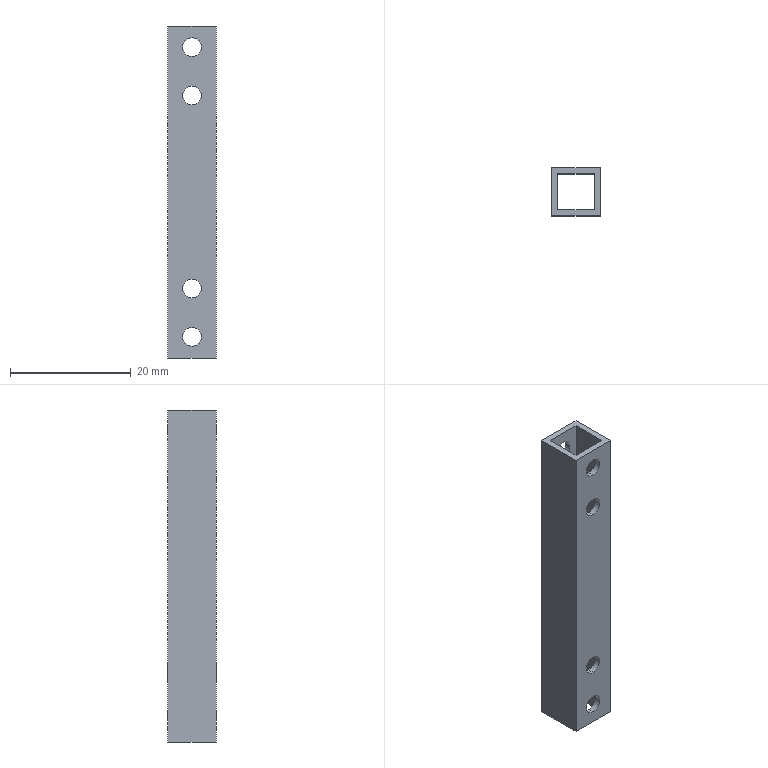Part | SolidWorks | features Extrusion 1, ICE 1 | 1 solid | 26 faces | box 8 x 8 x 55 mm | volume 1480 mm3 | cylinder 16 | plane 10 | commonest cylinder face diameters 3.1 x16
STEP:
#1=CARTESIAN_POINT('',(0.,3.,-5.05));
#2=VERTEX_POINT('',#1);
#3=CARTESIAN_POINT('',(0.,3.,-1.95));
#4=VERTEX_POINT('',#3);
#5=CARTESIAN_POINT('',(0.,3.,-3.5));
#6=DIRECTION('',(0.,1.,0.));
#7=DIRECTION('',(0.,0.,1.));
#8=AXIS2_PLACEMENT_3D('',#5,#6,#7);
#9=CIRCLE('',#8,1.55);
#10=EDGE_CURVE('',#2,#4,#9,.T.);
#11=ORIENTED_EDGE('',*,*,#10,.F.);
#12=CARTESIAN_POINT('',(0.,4.,-5.05));
#13=VERTEX_POINT('',#12);
#14=CARTESIAN_POINT('',(0.,-51.,-5.05));
#15=DIRECTION('',(0.,1.,0.));
#16=VECTOR('',#15,1000.);
#17=LINE('',#14,#16);
#18=EDGE_CURVE('',#2,#13,#17,.T.);
#19=ORIENTED_EDGE('',*,*,#18,.T.);
#20=CARTESIAN_POINT('',(0.,4.,-1.95));
#21=VERTEX_POINT('',#20);
#22=CARTESIAN_POINT('',(0.,4.,-3.5));
#23=DIRECTION('',(0.,1.,0.));
#24=DIRECTION('',(0.,0.,1.));
#25=AXIS2_PLACEMENT_3D('',#22,#23,#24);
#26=CIRCLE('',#25,1.55);
#27=EDGE_CURVE('',#13,#21,#26,.T.);
#28=ORIENTED_EDGE('',*,*,#27,.T.);
#29=CARTESIAN_POINT('',(0.,-51.,-1.95));
#30=DIRECTION('',(0.,1.,0.));
#31=VECTOR('',#30,1000.);
#32=LINE('',#29,#31);
#33=EDGE_CURVE('',#4,#21,#32,.T.);
#34=ORIENTED_EDGE('',*,*,#33,.F.);
#35=EDGE_LOOP('',(#11,#19,#28,#34));
#36=FACE_OUTER_BOUND('',#35,.T.);
#37=CARTESIAN_POINT('',(0.,-51.,-3.5));
#38=DIRECTION('',(0.,1.,0.));
#39=DIRECTION('',(0.,0.,1.));
#40=AXIS2_PLACEMENT_3D('',#37,#38,#39);
#41=CYLINDRICAL_SURFACE('',#40,1.55);
#42=ADVANCED_FACE('',(#36),#41,.F.);
#43=CARTESIAN_POINT('',(0.,3.,-13.05));
#44=VERTEX_POINT('',#43);
#45=CARTESIAN_POINT('',(0.,3.,-9.95));
#46=VERTEX_POINT('',#45);
#47=CARTESIAN_POINT('',(0.,3.,-11.5));
#48=DIRECTION('',(0.,1.,0.));
#49=DIRECTION('',(0.,0.,1.));
#50=AXIS2_PLACEMENT_3D('',#47,#48,#49);
#51=CIRCLE('',#50,1.55);
#52=EDGE_CURVE('',#44,#46,#51,.T.);
#53=ORIENTED_EDGE('',*,*,#52,.F.);
#54=CARTESIAN_POINT('',(0.,4.,-13.05));
#55=VERTEX_POINT('',#54);
#56=CARTESIAN_POINT('',(0.,-51.,-13.05));
#57=DIRECTION('',(0.,1.,0.));
#58=VECTOR('',#57,1000.);
#59=LINE('',#56,#58);
#60=EDGE_CURVE('',#44,#55,#59,.T.);
#61=ORIENTED_EDGE('',*,*,#60,.T.);
#62=CARTESIAN_POINT('',(0.,4.,-9.95));
#63=VERTEX_POINT('',#62);
#64=CARTESIAN_POINT('',(0.,4.,-11.5));
#65=DIRECTION('',(0.,1.,0.));
#66=DIRECTION('',(0.,0.,1.));
#67=AXIS2_PLACEMENT_3D('',#64,#65,#66);
#68=CIRCLE('',#67,1.55);
#69=EDGE_CURVE('',#55,#63,#68,.T.);
#70=ORIENTED_EDGE('',*,*,#69,.T.);
#71=CARTESIAN_POINT('',(0.,-51.,-9.95));
#72=DIRECTION('',(0.,1.,0.));
#73=VECTOR('',#72,1000.);
#74=LINE('',#71,#73);
#75=EDGE_CURVE('',#46,#63,#74,.T.);
#76=ORIENTED_EDGE('',*,*,#75,.F.);
#77=EDGE_LOOP('',(#53,#61,#70,#76));
#78=FACE_OUTER_BOUND('',#77,.T.);
#79=CARTESIAN_POINT('',(0.,-51.,-11.5));
#80=DIRECTION('',(0.,1.,0.));
#81=DIRECTION('',(0.,0.,1.));
#82=AXIS2_PLACEMENT_3D('',#79,#80,#81);
#83=CYLINDRICAL_SURFACE('',#82,1.55);
#84=ADVANCED_FACE('',(#78),#83,.F.);
#85=CARTESIAN_POINT('',(0.,3.,-45.05));
#86=VERTEX_POINT('',#85);
#87=CARTESIAN_POINT('',(0.,3.,-41.95));
#88=VERTEX_POINT('',#87);
#89=CARTESIAN_POINT('',(0.,3.,-43.5));
#90=DIRECTION('',(0.,1.,0.));
#91=DIRECTION('',(0.,0.,1.));
#92=AXIS2_PLACEMENT_3D('',#89,#90,#91);
#93=CIRCLE('',#92,1.55);
#94=EDGE_CURVE('',#86,#88,#93,.T.);
#95=ORIENTED_EDGE('',*,*,#94,.F.);
#96=CARTESIAN_POINT('',(0.,4.,-45.05));
#97=VERTEX_POINT('',#96);
#98=CARTESIAN_POINT('',(0.,-51.,-45.05));
#99=DIRECTION('',(0.,1.,0.));
#100=VECTOR('',#99,1000.);
#101=LINE('',#98,#100);
#102=EDGE_CURVE('',#86,#97,#101,.T.);
#103=ORIENTED_EDGE('',*,*,#102,.T.);
#104=CARTESIAN_POINT('',(0.,4.,-41.95));
#105=VERTEX_POINT('',#104);
#106=CARTESIAN_POINT('',(0.,4.,-43.5));
#107=DIRECTION('',(0.,1.,0.));
#108=DIRECTION('',(0.,0.,1.));
#109=AXIS2_PLACEMENT_3D('',#106,#107,#108);
#110=CIRCLE('',#109,1.55);
#111=EDGE_CURVE('',#97,#105,#110,.T.);
#112=ORIENTED_EDGE('',*,*,#111,.T.);
#113=CARTESIAN_POINT('',(0.,-51.,-41.95));
#114=DIRECTION('',(0.,1.,0.));
#115=VECTOR('',#114,1000.);
#116=LINE('',#113,#115);
#117=EDGE_CURVE('',#88,#105,#116,.T.);
#118=ORIENTED_EDGE('',*,*,#117,.F.);
#119=EDGE_LOOP('',(#95,#103,#112,#118));
#120=FACE_OUTER_BOUND('',#119,.T.);
#121=CARTESIAN_POINT('',(0.,-51.,-43.5));
#122=DIRECTION('',(0.,1.,0.));
#123=DIRECTION('',(0.,0.,1.));
#124=AXIS2_PLACEMENT_3D('',#121,#122,#123);
#125=CYLINDRICAL_SURFACE('',#124,1.55);
#126=ADVANCED_FACE('',(#120),#125,.F.);
#127=CARTESIAN_POINT('',(0.,3.,-53.05));
#128=VERTEX_POINT('',#127);
#129=CARTESIAN_POINT('',(0.,3.,-49.95));
#130=VERTEX_POINT('',#129);
#131=CARTESIAN_POINT('',(0.,3.,-51.5));
#132=DIRECTION('',(0.,1.,0.));
#133=DIRECTION('',(0.,0.,1.));
#134=AXIS2_PLACEMENT_3D('',#131,#132,#133);
#135=CIRCLE('',#134,1.55);
#136=EDGE_CURVE('',#128,#130,#135,.T.);
#137=ORIENTED_EDGE('',*,*,#136,.F.);
#138=CARTESIAN_POINT('',(0.,4.,-53.05));
#139=VERTEX_POINT('',#138);
#140=CARTESIAN_POINT('',(0.,-51.,-53.05));
#141=DIRECTION('',(0.,1.,0.));
#142=VECTOR('',#141,1000.);
#143=LINE('',#140,#142);
#144=EDGE_CURVE('',#128,#139,#143,.T.);
#145=ORIENTED_EDGE('',*,*,#144,.T.);
#146=CARTESIAN_POINT('',(0.,4.,-49.95));
#147=VERTEX_POINT('',#146);
#148=CARTESIAN_POINT('',(0.,4.,-51.5));
#149=DIRECTION('',(0.,1.,0.));
#150=DIRECTION('',(0.,0.,1.));
#151=AXIS2_PLACEMENT_3D('',#148,#149,#150);
#152=CIRCLE('',#151,1.55);
#153=EDGE_CURVE('',#139,#147,#152,.T.);
#154=ORIENTED_EDGE('',*,*,#153,.T.);
#155=CARTESIAN_POINT('',(0.,-51.,-49.95));
#156=DIRECTION('',(0.,1.,0.));
#157=VECTOR('',#156,1000.);
#158=LINE('',#155,#157);
#159=EDGE_CURVE('',#130,#147,#158,.T.);
#160=ORIENTED_EDGE('',*,*,#159,.F.);
#161=EDGE_LOOP('',(#137,#145,#154,#160));
#162=FACE_OUTER_BOUND('',#161,.T.);
#163=CARTESIAN_POINT('',(0.,-51.,-51.5));
#164=DIRECTION('',(0.,1.,0.));
#165=DIRECTION('',(0.,0.,1.));
#166=AXIS2_PLACEMENT_3D('',#163,#164,#165);
#167=CYLINDRICAL_SURFACE('',#166,1.55);
#168=ADVANCED_FACE('',(#162),#167,.F.);
#169=CARTESIAN_POINT('',(0.,-4.,-1.95));
#170=VERTEX_POINT('',#169);
#171=CARTESIAN_POINT('',(0.,-4.,-5.05));
#172=VERTEX_POINT('',#171);
#173=CARTESIAN_POINT('',(0.,-4.,-3.5));
#174=DIRECTION('',(0.,-1.,0.));
#175=DIRECTION('',(0.,0.,-1.));
#176=AXIS2_PLACEMENT_3D('',#173,#174,#175);
#177=CIRCLE('',#176,1.55);
#178=EDGE_CURVE('',#170,#172,#177,.T.);
#179=ORIENTED_EDGE('',*,*,#178,.T.);
#180=CARTESIAN_POINT('',(0.,-3.,-5.05));
#181=VERTEX_POINT('',#180);
#182=CARTESIAN_POINT('',(0.,-51.,-5.05));
#183=DIRECTION('',(0.,1.,0.));
#184=VECTOR('',#183,1000.);
#185=LINE('',#182,#184);
#186=EDGE_CURVE('',#172,#181,#185,.T.);
#187=ORIENTED_EDGE('',*,*,#186,.T.);
#188=CARTESIAN_POINT('',(0.,-3.,-1.95));
#189=VERTEX_POINT('',#188);
#190=CARTESIAN_POINT('',(0.,-3.,-3.5));
#191=DIRECTION('',(0.,-1.,0.));
#192=DIRECTION('',(0.,0.,-1.));
#193=AXIS2_PLACEMENT_3D('',#190,#191,#192);
#194=CIRCLE('',#193,1.55);
#195=EDGE_CURVE('',#189,#181,#194,.T.);
#196=ORIENTED_EDGE('',*,*,#195,.F.);
#197=CARTESIAN_POINT('',(0.,-51.,-1.95));
#198=DIRECTION('',(0.,1.,0.));
#199=VECTOR('',#198,1000.);
#200=LINE('',#197,#199);
#201=EDGE_CURVE('',#170,#189,#200,.T.);
#202=ORIENTED_EDGE('',*,*,#201,.F.);
#203=EDGE_LOOP('',(#179,#187,#196,#202));
#204=FACE_OUTER_BOUND('',#203,.T.);
#205=CARTESIAN_POINT('',(0.,-51.,-3.5));
#206=DIRECTION('',(0.,1.,0.));
#207=DIRECTION('',(0.,0.,1.));
#208=AXIS2_PLACEMENT_3D('',#205,#206,#207);
#209=CYLINDRICAL_SURFACE('',#208,1.55);
#210=ADVANCED_FACE('',(#204),#209,.F.);
#211=CARTESIAN_POINT('',(0.,-4.,-9.95));
#212=VERTEX_POINT('',#211);
#213=CARTESIAN_POINT('',(0.,-4.,-13.05));
#214=VERTEX_POINT('',#213);
#215=CARTESIAN_POINT('',(0.,-4.,-11.5));
#216=DIRECTION('',(0.,-1.,0.));
#217=DIRECTION('',(0.,0.,-1.));
#218=AXIS2_PLACEMENT_3D('',#215,#216,#217);
#219=CIRCLE('',#218,1.55);
#220=EDGE_CURVE('',#212,#214,#219,.T.);
#221=ORIENTED_EDGE('',*,*,#220,.T.);
#222=CARTESIAN_POINT('',(0.,-3.,-13.05));
#223=VERTEX_POINT('',#222);
#224=CARTESIAN_POINT('',(0.,-51.,-13.05));
#225=DIRECTION('',(0.,1.,0.));
#226=VECTOR('',#225,1000.);
#227=LINE('',#224,#226);
#228=EDGE_CURVE('',#214,#223,#227,.T.);
#229=ORIENTED_EDGE('',*,*,#228,.T.);
#230=CARTESIAN_POINT('',(0.,-3.,-9.95));
#231=VERTEX_POINT('',#230);
#232=CARTESIAN_POINT('',(0.,-3.,-11.5));
#233=DIRECTION('',(0.,-1.,0.));
#234=DIRECTION('',(0.,0.,-1.));
#235=AXIS2_PLACEMENT_3D('',#232,#233,#234);
#236=CIRCLE('',#235,1.55);
#237=EDGE_CURVE('',#231,#223,#236,.T.);
#238=ORIENTED_EDGE('',*,*,#237,.F.);
#239=CARTESIAN_POINT('',(0.,-51.,-9.95));
#240=DIRECTION('',(0.,1.,0.));
#241=VECTOR('',#240,1000.);
#242=LINE('',#239,#241);
#243=EDGE_CURVE('',#212,#231,#242,.T.);
#244=ORIENTED_EDGE('',*,*,#243,.F.);
#245=EDGE_LOOP('',(#221,#229,#238,#244));
#246=FACE_OUTER_BOUND('',#245,.T.);
#247=CARTESIAN_POINT('',(0.,-51.,-11.5));
#248=DIRECTION('',(0.,1.,0.));
#249=DIRECTION('',(0.,0.,1.));
#250=AXIS2_PLACEMENT_3D('',#247,#248,#249);
#251=CYLINDRICAL_SURFACE('',#250,1.55);
#252=ADVANCED_FACE('',(#246),#251,.F.);
#253=CARTESIAN_POINT('',(0.,-4.,-41.95));
#254=VERTEX_POINT('',#253);
#255=CARTESIAN_POINT('',(0.,-4.,-45.05));
#256=VERTEX_POINT('',#255);
#257=CARTESIAN_POINT('',(0.,-4.,-43.5));
#258=DIRECTION('',(0.,-1.,0.));
#259=DIRECTION('',(0.,0.,-1.));
#260=AXIS2_PLACEMENT_3D('',#257,#258,#259);
#261=CIRCLE('',#260,1.55);
#262=EDGE_CURVE('',#254,#256,#261,.T.);
#263=ORIENTED_EDGE('',*,*,#262,.T.);
#264=CARTESIAN_POINT('',(0.,-3.,-45.05));
#265=VERTEX_POINT('',#264);
#266=CARTESIAN_POINT('',(0.,-51.,-45.05));
#267=DIRECTION('',(0.,1.,0.));
#268=VECTOR('',#267,1000.);
#269=LINE('',#266,#268);
#270=EDGE_CURVE('',#256,#265,#269,.T.);
#271=ORIENTED_EDGE('',*,*,#270,.T.);
#272=CARTESIAN_POINT('',(0.,-3.,-41.95));
#273=VERTEX_POINT('',#272);
#274=CARTESIAN_POINT('',(0.,-3.,-43.5));
#275=DIRECTION('',(0.,-1.,0.));
#276=DIRECTION('',(0.,0.,-1.));
#277=AXIS2_PLACEMENT_3D('',#274,#275,#276);
#278=CIRCLE('',#277,1.55);
#279=EDGE_CURVE('',#273,#265,#278,.T.);
#280=ORIENTED_EDGE('',*,*,#279,.F.);
#281=CARTESIAN_POINT('',(0.,-51.,-41.95));
#282=DIRECTION('',(0.,1.,0.));
#283=VECTOR('',#282,1000.);
#284=LINE('',#281,#283);
#285=EDGE_CURVE('',#254,#273,#284,.T.);
#286=ORIENTED_EDGE('',*,*,#285,.F.);
#287=EDGE_LOOP('',(#263,#271,#280,#286));
#288=FACE_OUTER_BOUND('',#287,.T.);
#289=CARTESIAN_POINT('',(0.,-51.,-43.5));
#290=DIRECTION('',(0.,1.,0.));
#291=DIRECTION('',(0.,0.,1.));
#292=AXIS2_PLACEMENT_3D('',#289,#290,#291);
#293=CYLINDRICAL_SURFACE('',#292,1.55);
#294=ADVANCED_FACE('',(#288),#293,.F.);
#295=CARTESIAN_POINT('',(0.,-4.,-49.95));
#296=VERTEX_POINT('',#295);
#297=CARTESIAN_POINT('',(0.,-4.,-53.05));
#298=VERTEX_POINT('',#297);
#299=CARTESIAN_POINT('',(0.,-4.,-51.5));
#300=DIRECTION('',(0.,-1.,0.));
#301=DIRECTION('',(0.,0.,-1.));
#302=AXIS2_PLACEMENT_3D('',#299,#300,#301);
#303=CIRCLE('',#302,1.55);
#304=EDGE_CURVE('',#296,#298,#303,.T.);
#305=ORIENTED_EDGE('',*,*,#304,.T.);
#306=CARTESIAN_POINT('',(0.,-3.,-53.05));
#307=VERTEX_POINT('',#306);
#308=CARTESIAN_POINT('',(0.,-51.,-53.05));
#309=DIRECTION('',(0.,1.,0.));
#310=VECTOR('',#309,1000.);
#311=LINE('',#308,#310);
#312=EDGE_CURVE('',#298,#307,#311,.T.);
#313=ORIENTED_EDGE('',*,*,#312,.T.);
#314=CARTESIAN_POINT('',(0.,-3.,-49.95));
#315=VERTEX_POINT('',#314);
#316=CARTESIAN_POINT('',(0.,-3.,-51.5));
#317=DIRECTION('',(0.,-1.,0.));
#318=DIRECTION('',(0.,0.,-1.));
#319=AXIS2_PLACEMENT_3D('',#316,#317,#318);
#320=CIRCLE('',#319,1.55);
#321=EDGE_CURVE('',#315,#307,#320,.T.);
#322=ORIENTED_EDGE('',*,*,#321,.F.);
#323=CARTESIAN_POINT('',(0.,-51.,-49.95));
#324=DIRECTION('',(0.,1.,0.));
#325=VECTOR('',#324,1000.);
#326=LINE('',#323,#325);
#327=EDGE_CURVE('',#296,#315,#326,.T.);
#328=ORIENTED_EDGE('',*,*,#327,.F.);
#329=EDGE_LOOP('',(#305,#313,#322,#328));
#330=FACE_OUTER_BOUND('',#329,.T.);
#331=CARTESIAN_POINT('',(0.,-51.,-51.5));
#332=DIRECTION('',(0.,1.,0.));
#333=DIRECTION('',(0.,0.,1.));
#334=AXIS2_PLACEMENT_3D('',#331,#332,#333);
#335=CYLINDRICAL_SURFACE('',#334,1.55);
#336=ADVANCED_FACE('',(#330),#335,.F.);
#337=CARTESIAN_POINT('',(4.,-4.,0.));
#338=VERTEX_POINT('',#337);
#339=CARTESIAN_POINT('',(4.,4.,0.));
#340=VERTEX_POINT('',#339);
#341=CARTESIAN_POINT('',(4.,4.,0.));
#342=DIRECTION('',(0.,1.,0.));
#343=VECTOR('',#342,1000.);
#344=LINE('',#341,#343);
#345=EDGE_CURVE('',#338,#340,#344,.T.);
#346=ORIENTED_EDGE('',*,*,#345,.F.);
#347=CARTESIAN_POINT('',(4.,-4.,-55.));
#348=VERTEX_POINT('',#347);
#349=CARTESIAN_POINT('',(4.,-4.,-55.));
#350=DIRECTION('',(0.,0.,1.));
#351=VECTOR('',#350,1000.);
#352=LINE('',#349,#351);
#353=EDGE_CURVE('',#348,#338,#352,.T.);
#354=ORIENTED_EDGE('',*,*,#353,.F.);
#355=CARTESIAN_POINT('',(4.,4.,-55.));
#356=VERTEX_POINT('',#355);
#357=CARTESIAN_POINT('',(4.,4.,-55.));
#358=DIRECTION('',(0.,1.,0.));
#359=VECTOR('',#358,1000.);
#360=LINE('',#357,#359);
#361=EDGE_CURVE('',#348,#356,#360,.T.);
#362=ORIENTED_EDGE('',*,*,#361,.T.);
#363=CARTESIAN_POINT('',(4.,4.,-55.));
#364=DIRECTION('',(0.,0.,1.));
#365=VECTOR('',#364,1000.);
#366=LINE('',#363,#365);
#367=EDGE_CURVE('',#356,#340,#366,.T.);
#368=ORIENTED_EDGE('',*,*,#367,.T.);
#369=EDGE_LOOP('',(#346,#354,#362,#368));
#370=FACE_OUTER_BOUND('',#369,.T.);
#371=CARTESIAN_POINT('',(4.,4.,-55.));
#372=DIRECTION('',(1.,0.,0.));
#373=DIRECTION('',(0.,1.,0.));
#374=AXIS2_PLACEMENT_3D('',#371,#372,#373);
#375=PLANE('',#374);
#376=ADVANCED_FACE('',(#370),#375,.T.);
#377=ORIENTED_EDGE('',*,*,#178,.F.);
#378=CARTESIAN_POINT('',(0.,-4.,-3.5));
#379=DIRECTION('',(0.,-1.,0.));
#380=DIRECTION('',(0.,0.,-1.));
#381=AXIS2_PLACEMENT_3D('',#378,#379,#380);
#382=CIRCLE('',#381,1.55);
#383=EDGE_CURVE('',#172,#170,#382,.T.);
#384=ORIENTED_EDGE('',*,*,#383,.F.);
#385=EDGE_LOOP('',(#377,#384));
#386=FACE_BOUND('',#385,.T.);
#387=ORIENTED_EDGE('',*,*,#220,.F.);
#388=CARTESIAN_POINT('',(0.,-4.,-11.5));
#389=DIRECTION('',(0.,-1.,0.));
#390=DIRECTION('',(0.,0.,-1.));
#391=AXIS2_PLACEMENT_3D('',#388,#389,#390);
#392=CIRCLE('',#391,1.55);
#393=EDGE_CURVE('',#214,#212,#392,.T.);
#394=ORIENTED_EDGE('',*,*,#393,.F.);
#395=EDGE_LOOP('',(#387,#394));
#396=FACE_BOUND('',#395,.T.);
#397=ORIENTED_EDGE('',*,*,#262,.F.);
#398=CARTESIAN_POINT('',(0.,-4.,-43.5));
#399=DIRECTION('',(0.,-1.,0.));
#400=DIRECTION('',(0.,0.,-1.));
#401=AXIS2_PLACEMENT_3D('',#398,#399,#400);
#402=CIRCLE('',#401,1.55);
#403=EDGE_CURVE('',#256,#254,#402,.T.);
#404=ORIENTED_EDGE('',*,*,#403,.F.);
#405=EDGE_LOOP('',(#397,#404));
#406=FACE_BOUND('',#405,.T.);
#407=ORIENTED_EDGE('',*,*,#304,.F.);
#408=CARTESIAN_POINT('',(0.,-4.,-51.5));
#409=DIRECTION('',(0.,-1.,0.));
#410=DIRECTION('',(0.,0.,-1.));
#411=AXIS2_PLACEMENT_3D('',#408,#409,#410);
#412=CIRCLE('',#411,1.55);
#413=EDGE_CURVE('',#298,#296,#412,.T.);
#414=ORIENTED_EDGE('',*,*,#413,.F.);
#415=EDGE_LOOP('',(#407,#414));
#416=FACE_BOUND('',#415,.T.);
#417=CARTESIAN_POINT('',(-4.,-4.,0.));
#418=VERTEX_POINT('',#417);
#419=CARTESIAN_POINT('',(-4.,-4.,0.));
#420=DIRECTION('',(1.,0.,0.));
#421=VECTOR('',#420,1000.);
#422=LINE('',#419,#421);
#423=EDGE_CURVE('',#418,#338,#422,.T.);
#424=ORIENTED_EDGE('',*,*,#423,.F.);
#425=CARTESIAN_POINT('',(-4.,-4.,-55.));
#426=VERTEX_POINT('',#425);
#427=CARTESIAN_POINT('',(-4.,-4.,-55.));
#428=DIRECTION('',(0.,0.,1.));
#429=VECTOR('',#428,1000.);
#430=LINE('',#427,#429);
#431=EDGE_CURVE('',#426,#418,#430,.T.);
#432=ORIENTED_EDGE('',*,*,#431,.F.);
#433=CARTESIAN_POINT('',(-4.,-4.,-55.));
#434=DIRECTION('',(1.,0.,0.));
#435=VECTOR('',#434,1000.);
#436=LINE('',#433,#435);
#437=EDGE_CURVE('',#426,#348,#436,.T.);
#438=ORIENTED_EDGE('',*,*,#437,.T.);
#439=ORIENTED_EDGE('',*,*,#353,.T.);
#440=EDGE_LOOP('',(#424,#432,#438,#439));
#441=FACE_OUTER_BOUND('',#440,.T.);
#442=CARTESIAN_POINT('',(-4.,-4.,-55.));
#443=DIRECTION('',(0.,-1.,0.));
#444=DIRECTION('',(0.,0.,-1.));
#445=AXIS2_PLACEMENT_3D('',#442,#443,#444);
#446=PLANE('',#445);
#447=ADVANCED_FACE('',(#386,#396,#406,#416,#441),#446,.T.);
#448=CARTESIAN_POINT('',(-4.,4.,0.));
#449=VERTEX_POINT('',#448);
#450=CARTESIAN_POINT('',(-4.,4.,0.));
#451=DIRECTION('',(0.,-1.,0.));
#452=VECTOR('',#451,1000.);
#453=LINE('',#450,#452);
#454=EDGE_CURVE('',#449,#418,#453,.T.);
#455=ORIENTED_EDGE('',*,*,#454,.F.);
#456=CARTESIAN_POINT('',(-4.,4.,-55.));
#457=VERTEX_POINT('',#456);
#458=CARTESIAN_POINT('',(-4.,4.,-55.));
#459=DIRECTION('',(0.,0.,1.));
#460=VECTOR('',#459,1000.);
#461=LINE('',#458,#460);
#462=EDGE_CURVE('',#457,#449,#461,.T.);
#463=ORIENTED_EDGE('',*,*,#462,.F.);
#464=CARTESIAN_POINT('',(-4.,4.,-55.));
#465=DIRECTION('',(0.,-1.,0.));
#466=VECTOR('',#465,1000.);
#467=LINE('',#464,#466);
#468=EDGE_CURVE('',#457,#426,#467,.T.);
#469=ORIENTED_EDGE('',*,*,#468,.T.);
#470=ORIENTED_EDGE('',*,*,#431,.T.);
#471=EDGE_LOOP('',(#455,#463,#469,#470));
#472=FACE_OUTER_BOUND('',#471,.T.);
#473=CARTESIAN_POINT('',(-4.,4.,-55.));
#474=DIRECTION('',(-1.,0.,0.));
#475=DIRECTION('',(0.,-1.,0.));
#476=AXIS2_PLACEMENT_3D('',#473,#474,#475);
#477=PLANE('',#476);
#478=ADVANCED_FACE('',(#472),#477,.T.);
#479=CARTESIAN_POINT('',(0.,4.,-3.5));
#480=DIRECTION('',(0.,1.,0.));
#481=DIRECTION('',(0.,0.,1.));
#482=AXIS2_PLACEMENT_3D('',#479,#480,#481);
#483=CIRCLE('',#482,1.55);
#484=EDGE_CURVE('',#21,#13,#483,.T.);
#485=ORIENTED_EDGE('',*,*,#484,.F.);
#486=ORIENTED_EDGE('',*,*,#27,.F.);
#487=EDGE_LOOP('',(#485,#486));
#488=FACE_BOUND('',#487,.T.);
#489=CARTESIAN_POINT('',(0.,4.,-11.5));
#490=DIRECTION('',(0.,1.,0.));
#491=DIRECTION('',(0.,0.,1.));
#492=AXIS2_PLACEMENT_3D('',#489,#490,#491);
#493=CIRCLE('',#492,1.55);
#494=EDGE_CURVE('',#63,#55,#493,.T.);
#495=ORIENTED_EDGE('',*,*,#494,.F.);
#496=ORIENTED_EDGE('',*,*,#69,.F.);
#497=EDGE_LOOP('',(#495,#496));
#498=FACE_BOUND('',#497,.T.);
#499=CARTESIAN_POINT('',(0.,4.,-43.5));
#500=DIRECTION('',(0.,1.,0.));
#501=DIRECTION('',(0.,0.,1.));
#502=AXIS2_PLACEMENT_3D('',#499,#500,#501);
#503=CIRCLE('',#502,1.55);
#504=EDGE_CURVE('',#105,#97,#503,.T.);
#505=ORIENTED_EDGE('',*,*,#504,.F.);
#506=ORIENTED_EDGE('',*,*,#111,.F.);
#507=EDGE_LOOP('',(#505,#506));
#508=FACE_BOUND('',#507,.T.);
#509=CARTESIAN_POINT('',(0.,4.,-51.5));
#510=DIRECTION('',(0.,1.,0.));
#511=DIRECTION('',(0.,0.,1.));
#512=AXIS2_PLACEMENT_3D('',#509,#510,#511);
#513=CIRCLE('',#512,1.55);
#514=EDGE_CURVE('',#147,#139,#513,.T.);
#515=ORIENTED_EDGE('',*,*,#514,.F.);
#516=ORIENTED_EDGE('',*,*,#153,.F.);
#517=EDGE_LOOP('',(#515,#516));
#518=FACE_BOUND('',#517,.T.);
#519=CARTESIAN_POINT('',(-4.,4.,0.));
#520=DIRECTION('',(-1.,0.,0.));
#521=VECTOR('',#520,1000.);
#522=LINE('',#519,#521);
#523=EDGE_CURVE('',#340,#449,#522,.T.);
#524=ORIENTED_EDGE('',*,*,#523,.F.);
#525=ORIENTED_EDGE('',*,*,#367,.F.);
#526=CARTESIAN_POINT('',(-4.,4.,-55.));
#527=DIRECTION('',(-1.,0.,0.));
#528=VECTOR('',#527,1000.);
#529=LINE('',#526,#528);
#530=EDGE_CURVE('',#356,#457,#529,.T.);
#531=ORIENTED_EDGE('',*,*,#530,.T.);
#532=ORIENTED_EDGE('',*,*,#462,.T.);
#533=EDGE_LOOP('',(#524,#525,#531,#532));
#534=FACE_OUTER_BOUND('',#533,.T.);
#535=CARTESIAN_POINT('',(-4.,4.,-55.));
#536=DIRECTION('',(0.,1.,0.));
#537=DIRECTION('',(0.,0.,1.));
#538=AXIS2_PLACEMENT_3D('',#535,#536,#537);
#539=PLANE('',#538);
#540=ADVANCED_FACE('',(#488,#498,#508,#518,#534),#539,.T.);
#541=CARTESIAN_POINT('',(3.,3.,-55.));
#542=VERTEX_POINT('',#541);
#543=CARTESIAN_POINT('',(-3.,3.,-55.));
#544=VERTEX_POINT('',#543);
#545=CARTESIAN_POINT('',(-3.,3.,-55.));
#546=DIRECTION('',(-1.,0.,0.));
#547=VECTOR('',#546,1000.);
#548=LINE('',#545,#547);
#549=EDGE_CURVE('',#542,#544,#548,.T.);
#550=ORIENTED_EDGE('',*,*,#549,.T.);
#551=CARTESIAN_POINT('',(-3.,-3.,-55.));
#552=VERTEX_POINT('',#551);
#553=CARTESIAN_POINT('',(-3.,3.,-55.));
#554=DIRECTION('',(0.,-1.,0.));
#555=VECTOR('',#554,1000.);
#556=LINE('',#553,#555);
#557=EDGE_CURVE('',#544,#552,#556,.T.);
#558=ORIENTED_EDGE('',*,*,#557,.T.);
#559=CARTESIAN_POINT('',(3.,-3.,-55.));
#560=VERTEX_POINT('',#559);
#561=CARTESIAN_POINT('',(-3.,-3.,-55.));
#562=DIRECTION('',(1.,0.,0.));
#563=VECTOR('',#562,1000.);
#564=LINE('',#561,#563);
#565=EDGE_CURVE('',#552,#560,#564,.T.);
#566=ORIENTED_EDGE('',*,*,#565,.T.);
#567=CARTESIAN_POINT('',(3.,3.,-55.));
#568=DIRECTION('',(0.,1.,0.));
#569=VECTOR('',#568,1000.);
#570=LINE('',#567,#569);
#571=EDGE_CURVE('',#560,#542,#570,.T.);
#572=ORIENTED_EDGE('',*,*,#571,.T.);
#573=EDGE_LOOP('',(#550,#558,#566,#572));
#574=FACE_BOUND('',#573,.T.);
#575=ORIENTED_EDGE('',*,*,#361,.F.);
#576=ORIENTED_EDGE('',*,*,#437,.F.);
#577=ORIENTED_EDGE('',*,*,#468,.F.);
#578=ORIENTED_EDGE('',*,*,#530,.F.);
#579=EDGE_LOOP('',(#575,#576,#577,#578));
#580=FACE_OUTER_BOUND('',#579,.T.);
#581=CARTESIAN_POINT('',(0.,0.,-55.));
#582=DIRECTION('',(0.,0.,1.));
#583=DIRECTION('',(1.,0.,0.));
#584=AXIS2_PLACEMENT_3D('',#581,#582,#583);
#585=PLANE('',#584);
#586=ADVANCED_FACE('',(#574,#580),#585,.F.);
#587=CARTESIAN_POINT('',(-3.,3.,0.));
#588=VERTEX_POINT('',#587);
#589=CARTESIAN_POINT('',(-3.,-3.,0.));
#590=VERTEX_POINT('',#589);
#591=CARTESIAN_POINT('',(-3.,3.,0.));
#592=DIRECTION('',(0.,-1.,0.));
#593=VECTOR('',#592,1000.);
#594=LINE('',#591,#593);
#595=EDGE_CURVE('',#588,#590,#594,.T.);
#596=ORIENTED_EDGE('',*,*,#595,.F.);
#597=CARTESIAN_POINT('',(3.,3.,0.));
#598=VERTEX_POINT('',#597);
#599=CARTESIAN_POINT('',(-3.,3.,0.));
#600=DIRECTION('',(-1.,0.,0.));
#601=VECTOR('',#600,1000.);
#602=LINE('',#599,#601);
#603=EDGE_CURVE('',#598,#588,#602,.T.);
#604=ORIENTED_EDGE('',*,*,#603,.F.);
#605=CARTESIAN_POINT('',(3.,-3.,0.));
#606=VERTEX_POINT('',#605);
#607=CARTESIAN_POINT('',(3.,3.,0.));
#608=DIRECTION('',(0.,1.,0.));
#609=VECTOR('',#608,1000.);
#610=LINE('',#607,#609);
#611=EDGE_CURVE('',#606,#598,#610,.T.);
#612=ORIENTED_EDGE('',*,*,#611,.F.);
#613=CARTESIAN_POINT('',(-3.,-3.,0.));
#614=DIRECTION('',(1.,0.,0.));
#615=VECTOR('',#614,1000.);
#616=LINE('',#613,#615);
#617=EDGE_CURVE('',#590,#606,#616,.T.);
#618=ORIENTED_EDGE('',*,*,#617,.F.);
#619=EDGE_LOOP('',(#596,#604,#612,#618));
#620=FACE_BOUND('',#619,.T.);
#621=ORIENTED_EDGE('',*,*,#345,.T.);
#622=ORIENTED_EDGE('',*,*,#523,.T.);
#623=ORIENTED_EDGE('',*,*,#454,.T.);
#624=ORIENTED_EDGE('',*,*,#423,.T.);
#625=EDGE_LOOP('',(#621,#622,#623,#624));
#626=FACE_OUTER_BOUND('',#625,.T.);
#627=CARTESIAN_POINT('',(0.,0.,0.));
#628=DIRECTION('',(0.,0.,1.));
#629=DIRECTION('',(1.,0.,0.));
#630=AXIS2_PLACEMENT_3D('',#627,#628,#629);
#631=PLANE('',#630);
#632=ADVANCED_FACE('',(#620,#626),#631,.T.);
#633=ORIENTED_EDGE('',*,*,#595,.T.);
#634=CARTESIAN_POINT('',(-3.,-3.,-55.));
#635=DIRECTION('',(0.,0.,1.));
#636=VECTOR('',#635,1000.);
#637=LINE('',#634,#636);
#638=EDGE_CURVE('',#552,#590,#637,.T.);
#639=ORIENTED_EDGE('',*,*,#638,.F.);
#640=ORIENTED_EDGE('',*,*,#557,.F.);
#641=CARTESIAN_POINT('',(-3.,3.,-55.));
#642=DIRECTION('',(0.,0.,1.));
#643=VECTOR('',#642,1000.);
#644=LINE('',#641,#643);
#645=EDGE_CURVE('',#544,#588,#644,.T.);
#646=ORIENTED_EDGE('',*,*,#645,.T.);
#647=EDGE_LOOP('',(#633,#639,#640,#646));
#648=FACE_OUTER_BOUND('',#647,.T.);
#649=CARTESIAN_POINT('',(-3.,3.,-55.));
#650=DIRECTION('',(-1.,0.,0.));
#651=DIRECTION('',(0.,0.,1.));
#652=AXIS2_PLACEMENT_3D('',#649,#650,#651);
#653=PLANE('',#652);
#654=ADVANCED_FACE('',(#648),#653,.F.);
#655=CARTESIAN_POINT('',(0.,3.,-3.5));
#656=DIRECTION('',(0.,1.,0.));
#657=DIRECTION('',(0.,0.,1.));
#658=AXIS2_PLACEMENT_3D('',#655,#656,#657);
#659=CIRCLE('',#658,1.55);
#660=EDGE_CURVE('',#4,#2,#659,.T.);
#661=ORIENTED_EDGE('',*,*,#660,.T.);
#662=ORIENTED_EDGE('',*,*,#10,.T.);
#663=EDGE_LOOP('',(#661,#662));
#664=FACE_BOUND('',#663,.T.);
#665=CARTESIAN_POINT('',(0.,3.,-11.5));
#666=DIRECTION('',(0.,1.,0.));
#667=DIRECTION('',(0.,0.,1.));
#668=AXIS2_PLACEMENT_3D('',#665,#666,#667);
#669=CIRCLE('',#668,1.55);
#670=EDGE_CURVE('',#46,#44,#669,.T.);
#671=ORIENTED_EDGE('',*,*,#670,.T.);
#672=ORIENTED_EDGE('',*,*,#52,.T.);
#673=EDGE_LOOP('',(#671,#672));
#674=FACE_BOUND('',#673,.T.);
#675=CARTESIAN_POINT('',(0.,3.,-43.5));
#676=DIRECTION('',(0.,1.,0.));
#677=DIRECTION('',(0.,0.,1.));
#678=AXIS2_PLACEMENT_3D('',#675,#676,#677);
#679=CIRCLE('',#678,1.55);
#680=EDGE_CURVE('',#88,#86,#679,.T.);
#681=ORIENTED_EDGE('',*,*,#680,.T.);
#682=ORIENTED_EDGE('',*,*,#94,.T.);
#683=EDGE_LOOP('',(#681,#682));
#684=FACE_BOUND('',#683,.T.);
#685=CARTESIAN_POINT('',(0.,3.,-51.5));
#686=DIRECTION('',(0.,1.,0.));
#687=DIRECTION('',(0.,0.,1.));
#688=AXIS2_PLACEMENT_3D('',#685,#686,#687);
#689=CIRCLE('',#688,1.55);
#690=EDGE_CURVE('',#130,#128,#689,.T.);
#691=ORIENTED_EDGE('',*,*,#690,.T.);
#692=ORIENTED_EDGE('',*,*,#136,.T.);
#693=EDGE_LOOP('',(#691,#692));
#694=FACE_BOUND('',#693,.T.);
#695=ORIENTED_EDGE('',*,*,#603,.T.);
#696=ORIENTED_EDGE('',*,*,#645,.F.);
#697=ORIENTED_EDGE('',*,*,#549,.F.);
#698=CARTESIAN_POINT('',(3.,3.,-55.));
#699=DIRECTION('',(0.,0.,1.));
#700=VECTOR('',#699,1000.);
#701=LINE('',#698,#700);
#702=EDGE_CURVE('',#542,#598,#701,.T.);
#703=ORIENTED_EDGE('',*,*,#702,.T.);
#704=EDGE_LOOP('',(#695,#696,#697,#703));
#705=FACE_OUTER_BOUND('',#704,.T.);
#706=CARTESIAN_POINT('',(-3.,3.,-55.));
#707=DIRECTION('',(0.,1.,0.));
#708=DIRECTION('',(0.,0.,1.));
#709=AXIS2_PLACEMENT_3D('',#706,#707,#708);
#710=PLANE('',#709);
#711=ADVANCED_FACE('',(#664,#674,#684,#694,#705),#710,.F.);
#712=ORIENTED_EDGE('',*,*,#611,.T.);
#713=ORIENTED_EDGE('',*,*,#702,.F.);
#714=ORIENTED_EDGE('',*,*,#571,.F.);
#715=CARTESIAN_POINT('',(3.,-3.,-55.));
#716=DIRECTION('',(0.,0.,1.));
#717=VECTOR('',#716,1000.);
#718=LINE('',#715,#717);
#719=EDGE_CURVE('',#560,#606,#718,.T.);
#720=ORIENTED_EDGE('',*,*,#719,.T.);
#721=EDGE_LOOP('',(#712,#713,#714,#720));
#722=FACE_OUTER_BOUND('',#721,.T.);
#723=CARTESIAN_POINT('',(3.,3.,-55.));
#724=DIRECTION('',(1.,0.,0.));
#725=DIRECTION('',(0.,0.,-1.));
#726=AXIS2_PLACEMENT_3D('',#723,#724,#725);
#727=PLANE('',#726);
#728=ADVANCED_FACE('',(#722),#727,.F.);
#729=ORIENTED_EDGE('',*,*,#195,.T.);
#730=CARTESIAN_POINT('',(0.,-3.,-3.5));
#731=DIRECTION('',(0.,-1.,0.));
#732=DIRECTION('',(0.,0.,-1.));
#733=AXIS2_PLACEMENT_3D('',#730,#731,#732);
#734=CIRCLE('',#733,1.55);
#735=EDGE_CURVE('',#181,#189,#734,.T.);
#736=ORIENTED_EDGE('',*,*,#735,.T.);
#737=EDGE_LOOP('',(#729,#736));
#738=FACE_BOUND('',#737,.T.);
#739=ORIENTED_EDGE('',*,*,#237,.T.);
#740=CARTESIAN_POINT('',(0.,-3.,-11.5));
#741=DIRECTION('',(0.,-1.,0.));
#742=DIRECTION('',(0.,0.,-1.));
#743=AXIS2_PLACEMENT_3D('',#740,#741,#742);
#744=CIRCLE('',#743,1.55);
#745=EDGE_CURVE('',#223,#231,#744,.T.);
#746=ORIENTED_EDGE('',*,*,#745,.T.);
#747=EDGE_LOOP('',(#739,#746));
#748=FACE_BOUND('',#747,.T.);
#749=ORIENTED_EDGE('',*,*,#279,.T.);
#750=CARTESIAN_POINT('',(0.,-3.,-43.5));
#751=DIRECTION('',(0.,-1.,0.));
#752=DIRECTION('',(0.,0.,-1.));
#753=AXIS2_PLACEMENT_3D('',#750,#751,#752);
#754=CIRCLE('',#753,1.55);
#755=EDGE_CURVE('',#265,#273,#754,.T.);
#756=ORIENTED_EDGE('',*,*,#755,.T.);
#757=EDGE_LOOP('',(#749,#756));
#758=FACE_BOUND('',#757,.T.);
#759=ORIENTED_EDGE('',*,*,#321,.T.);
#760=CARTESIAN_POINT('',(0.,-3.,-51.5));
#761=DIRECTION('',(0.,-1.,0.));
#762=DIRECTION('',(0.,0.,-1.));
#763=AXIS2_PLACEMENT_3D('',#760,#761,#762);
#764=CIRCLE('',#763,1.55);
#765=EDGE_CURVE('',#307,#315,#764,.T.);
#766=ORIENTED_EDGE('',*,*,#765,.T.);
#767=EDGE_LOOP('',(#759,#766));
#768=FACE_BOUND('',#767,.T.);
#769=ORIENTED_EDGE('',*,*,#617,.T.);
#770=ORIENTED_EDGE('',*,*,#719,.F.);
#771=ORIENTED_EDGE('',*,*,#565,.F.);
#772=ORIENTED_EDGE('',*,*,#638,.T.);
#773=EDGE_LOOP('',(#769,#770,#771,#772));
#774=FACE_OUTER_BOUND('',#773,.T.);
#775=CARTESIAN_POINT('',(-3.,-3.,-55.));
#776=DIRECTION('',(0.,-1.,0.));
#777=DIRECTION('',(0.,0.,-1.));
#778=AXIS2_PLACEMENT_3D('',#775,#776,#777);
#779=PLANE('',#778);
#780=ADVANCED_FACE('',(#738,#748,#758,#768,#774),#779,.F.);
#781=ORIENTED_EDGE('',*,*,#312,.F.);
#782=ORIENTED_EDGE('',*,*,#413,.T.);
#783=ORIENTED_EDGE('',*,*,#327,.T.);
#784=ORIENTED_EDGE('',*,*,#765,.F.);
#785=EDGE_LOOP('',(#781,#782,#783,#784));
#786=FACE_OUTER_BOUND('',#785,.T.);
#787=CARTESIAN_POINT('',(0.,-51.,-51.5));
#788=DIRECTION('',(0.,1.,0.));
#789=DIRECTION('',(0.,0.,1.));
#790=AXIS2_PLACEMENT_3D('',#787,#788,#789);
#791=CYLINDRICAL_SURFACE('',#790,1.55);
#792=ADVANCED_FACE('',(#786),#791,.F.);
#793=ORIENTED_EDGE('',*,*,#270,.F.);
#794=ORIENTED_EDGE('',*,*,#403,.T.);
#795=ORIENTED_EDGE('',*,*,#285,.T.);
#796=ORIENTED_EDGE('',*,*,#755,.F.);
#797=EDGE_LOOP('',(#793,#794,#795,#796));
#798=FACE_OUTER_BOUND('',#797,.T.);
#799=CARTESIAN_POINT('',(0.,-51.,-43.5));
#800=DIRECTION('',(0.,1.,0.));
#801=DIRECTION('',(0.,0.,1.));
#802=AXIS2_PLACEMENT_3D('',#799,#800,#801);
#803=CYLINDRICAL_SURFACE('',#802,1.55);
#804=ADVANCED_FACE('',(#798),#803,.F.);
#805=ORIENTED_EDGE('',*,*,#228,.F.);
#806=ORIENTED_EDGE('',*,*,#393,.T.);
#807=ORIENTED_EDGE('',*,*,#243,.T.);
#808=ORIENTED_EDGE('',*,*,#745,.F.);
#809=EDGE_LOOP('',(#805,#806,#807,#808));
#810=FACE_OUTER_BOUND('',#809,.T.);
#811=CARTESIAN_POINT('',(0.,-51.,-11.5));
#812=DIRECTION('',(0.,1.,0.));
#813=DIRECTION('',(0.,0.,1.));
#814=AXIS2_PLACEMENT_3D('',#811,#812,#813);
#815=CYLINDRICAL_SURFACE('',#814,1.55);
#816=ADVANCED_FACE('',(#810),#815,.F.);
#817=ORIENTED_EDGE('',*,*,#186,.F.);
#818=ORIENTED_EDGE('',*,*,#383,.T.);
#819=ORIENTED_EDGE('',*,*,#201,.T.);
#820=ORIENTED_EDGE('',*,*,#735,.F.);
#821=EDGE_LOOP('',(#817,#818,#819,#820));
#822=FACE_OUTER_BOUND('',#821,.T.);
#823=CARTESIAN_POINT('',(0.,-51.,-3.5));
#824=DIRECTION('',(0.,1.,0.));
#825=DIRECTION('',(0.,0.,1.));
#826=AXIS2_PLACEMENT_3D('',#823,#824,#825);
#827=CYLINDRICAL_SURFACE('',#826,1.55);
#828=ADVANCED_FACE('',(#822),#827,.F.);
#829=ORIENTED_EDGE('',*,*,#144,.F.);
#830=ORIENTED_EDGE('',*,*,#690,.F.);
#831=ORIENTED_EDGE('',*,*,#159,.T.);
#832=ORIENTED_EDGE('',*,*,#514,.T.);
#833=EDGE_LOOP('',(#829,#830,#831,#832));
#834=FACE_OUTER_BOUND('',#833,.T.);
#835=CARTESIAN_POINT('',(0.,-51.,-51.5));
#836=DIRECTION('',(0.,1.,0.));
#837=DIRECTION('',(0.,0.,1.));
#838=AXIS2_PLACEMENT_3D('',#835,#836,#837);
#839=CYLINDRICAL_SURFACE('',#838,1.55);
#840=ADVANCED_FACE('',(#834),#839,.F.);
#841=ORIENTED_EDGE('',*,*,#102,.F.);
#842=ORIENTED_EDGE('',*,*,#680,.F.);
#843=ORIENTED_EDGE('',*,*,#117,.T.);
#844=ORIENTED_EDGE('',*,*,#504,.T.);
#845=EDGE_LOOP('',(#841,#842,#843,#844));
#846=FACE_OUTER_BOUND('',#845,.T.);
#847=CARTESIAN_POINT('',(0.,-51.,-43.5));
#848=DIRECTION('',(0.,1.,0.));
#849=DIRECTION('',(0.,0.,1.));
#850=AXIS2_PLACEMENT_3D('',#847,#848,#849);
#851=CYLINDRICAL_SURFACE('',#850,1.55);
#852=ADVANCED_FACE('',(#846),#851,.F.);
#853=ORIENTED_EDGE('',*,*,#60,.F.);
#854=ORIENTED_EDGE('',*,*,#670,.F.);
#855=ORIENTED_EDGE('',*,*,#75,.T.);
#856=ORIENTED_EDGE('',*,*,#494,.T.);
#857=EDGE_LOOP('',(#853,#854,#855,#856));
#858=FACE_OUTER_BOUND('',#857,.T.);
#859=CARTESIAN_POINT('',(0.,-51.,-11.5));
#860=DIRECTION('',(0.,1.,0.));
#861=DIRECTION('',(0.,0.,1.));
#862=AXIS2_PLACEMENT_3D('',#859,#860,#861);
#863=CYLINDRICAL_SURFACE('',#862,1.55);
#864=ADVANCED_FACE('',(#858),#863,.F.);
#865=ORIENTED_EDGE('',*,*,#18,.F.);
#866=ORIENTED_EDGE('',*,*,#660,.F.);
#867=ORIENTED_EDGE('',*,*,#33,.T.);
#868=ORIENTED_EDGE('',*,*,#484,.T.);
#869=EDGE_LOOP('',(#865,#866,#867,#868));
#870=FACE_OUTER_BOUND('',#869,.T.);
#871=CARTESIAN_POINT('',(0.,-51.,-3.5));
#872=DIRECTION('',(0.,1.,0.));
#873=DIRECTION('',(0.,0.,1.));
#874=AXIS2_PLACEMENT_3D('',#871,#872,#873);
#875=CYLINDRICAL_SURFACE('',#874,1.55);
#876=ADVANCED_FACE('',(#870),#875,.F.);
#877=CLOSED_SHELL('',(#42,#84,#126,#168,#210,#252,#294,#336,#376,#447,#478,#540,#586,#632,#654,#711,#728,#780,#792,#804,#816,#828,#840,#852,#864,#876));
#878=MANIFOLD_SOLID_BREP('',#877);
#879=CARTESIAN_POINT('',(0.,0.,0.));
#880=DIRECTION('',(0.,0.,1.));
#881=DIRECTION('',(1.,0.,0.));
#882=AXIS2_PLACEMENT_3D('',#879,#880,#881);
#883=(LENGTH_UNIT()NAMED_UNIT(*)SI_UNIT(.MILLI.,.METRE.));
#884=UNCERTAINTY_MEASURE_WITH_UNIT(LENGTH_MEASURE(0.00001),#883,'','');
#885=(NAMED_UNIT(*)PLANE_ANGLE_UNIT()SI_UNIT($,.RADIAN.));
#886=(NAMED_UNIT(*)SI_UNIT($,.STERADIAN.)SOLID_ANGLE_UNIT());
#887=(GEOMETRIC_REPRESENTATION_CONTEXT(3)GLOBAL_UNCERTAINTY_ASSIGNED_CONTEXT((#884))GLOBAL_UNIT_ASSIGNED_CONTEXT((#883,#885,#886))REPRESENTATION_CONTEXT('',''));
#888=ADVANCED_BREP_SHAPE_REPRESENTATION('',(#878,#882),#887);